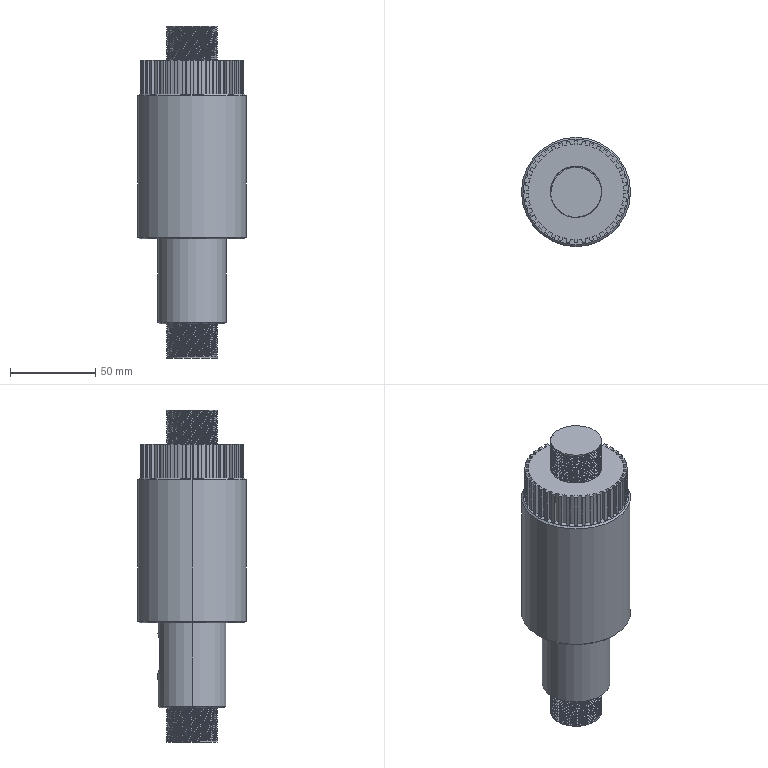Part | SolidWorks | features ICE 5, SweepThread 2, Chamfer 1, Extrusion 1 | 1 solid | 273 faces | box 64 x 64 x 195 mm | volume 414709 mm3 | cylinder 166 | plane 93 | spline 8 | cone 6 | commonest cylinder face diameters 30 x78 60 x41 55.985 x40 12 x3 40 x2 64 x2